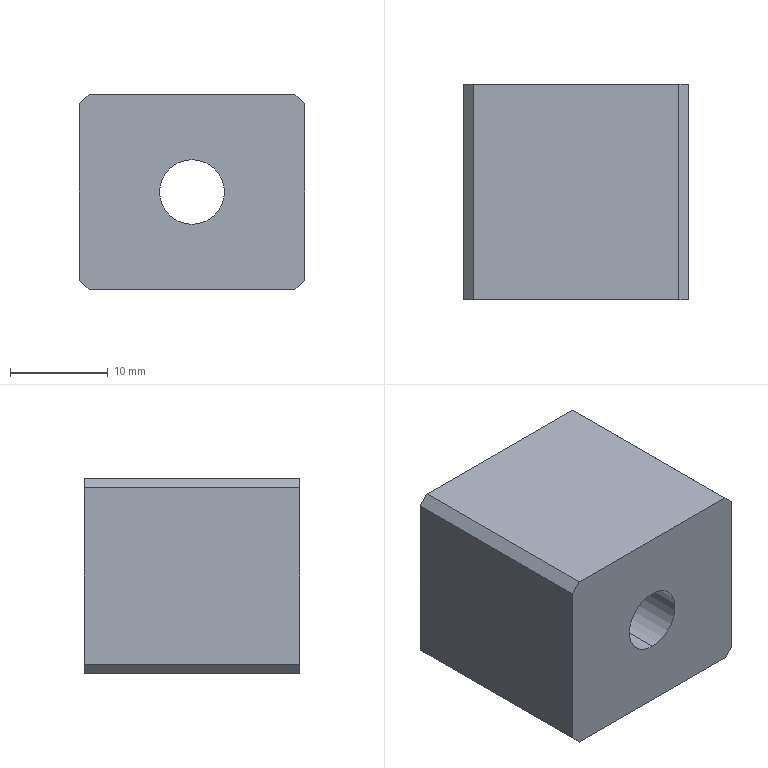Part | SolidWorks | features Chamfer 1, Extrusion 1, HoleWzd 1 | 1 solid | 15 faces | box 23 x 22 x 20 mm | volume 8934 mm3 | plane 11 | cylinder 4 | commonest cylinder face diameters 6.6 x2 11 x2
STEP:
#1=CARTESIAN_POINT('',(0.,4.6,-5.5));
#2=VERTEX_POINT('',#1);
#3=CARTESIAN_POINT('',(0.,4.6,5.5));
#4=VERTEX_POINT('',#3);
#5=CARTESIAN_POINT('',(0.,4.6,0.));
#6=DIRECTION('',(0.,1.,0.));
#7=DIRECTION('',(0.,0.,1.));
#8=AXIS2_PLACEMENT_3D('',#5,#6,#7);
#9=CIRCLE('',#8,5.5);
#10=EDGE_CURVE('',#2,#4,#9,.T.);
#11=ORIENTED_EDGE('',*,*,#10,.F.);
#12=CARTESIAN_POINT('',(0.,11.,-5.5));
#13=VERTEX_POINT('',#12);
#14=CARTESIAN_POINT('',(0.,11.,-5.5));
#15=DIRECTION('',(0.,1.,0.));
#16=VECTOR('',#15,1000.);
#17=LINE('',#14,#16);
#18=EDGE_CURVE('',#2,#13,#17,.T.);
#19=ORIENTED_EDGE('',*,*,#18,.T.);
#20=CARTESIAN_POINT('',(0.,11.,5.5));
#21=VERTEX_POINT('',#20);
#22=CARTESIAN_POINT('',(0.,11.,0.));
#23=DIRECTION('',(0.,1.,0.));
#24=DIRECTION('',(0.,0.,1.));
#25=AXIS2_PLACEMENT_3D('',#22,#23,#24);
#26=CIRCLE('',#25,5.5);
#27=EDGE_CURVE('',#13,#21,#26,.T.);
#28=ORIENTED_EDGE('',*,*,#27,.T.);
#29=CARTESIAN_POINT('',(0.,11.,5.5));
#30=DIRECTION('',(0.,1.,0.));
#31=VECTOR('',#30,1000.);
#32=LINE('',#29,#31);
#33=EDGE_CURVE('',#4,#21,#32,.T.);
#34=ORIENTED_EDGE('',*,*,#33,.F.);
#35=EDGE_LOOP('',(#11,#19,#28,#34));
#36=FACE_OUTER_BOUND('',#35,.T.);
#37=CARTESIAN_POINT('',(0.,11.,0.));
#38=DIRECTION('',(0.,1.,0.));
#39=DIRECTION('',(0.,0.,1.));
#40=AXIS2_PLACEMENT_3D('',#37,#38,#39);
#41=CYLINDRICAL_SURFACE('',#40,5.5);
#42=ADVANCED_FACE('',(#36),#41,.F.);
#43=CARTESIAN_POINT('',(0.,-11.,-3.3));
#44=VERTEX_POINT('',#43);
#45=CARTESIAN_POINT('',(0.,-11.,3.3));
#46=VERTEX_POINT('',#45);
#47=CARTESIAN_POINT('',(0.,-11.,0.));
#48=DIRECTION('',(0.,1.,0.));
#49=DIRECTION('',(0.,0.,1.));
#50=AXIS2_PLACEMENT_3D('',#47,#48,#49);
#51=CIRCLE('',#50,3.3);
#52=EDGE_CURVE('',#44,#46,#51,.T.);
#53=ORIENTED_EDGE('',*,*,#52,.F.);
#54=CARTESIAN_POINT('',(0.,4.6,-3.3));
#55=VERTEX_POINT('',#54);
#56=CARTESIAN_POINT('',(0.,11.,-3.3));
#57=DIRECTION('',(0.,1.,0.));
#58=VECTOR('',#57,1000.);
#59=LINE('',#56,#58);
#60=EDGE_CURVE('',#44,#55,#59,.T.);
#61=ORIENTED_EDGE('',*,*,#60,.T.);
#62=CARTESIAN_POINT('',(0.,4.6,3.3));
#63=VERTEX_POINT('',#62);
#64=CARTESIAN_POINT('',(0.,4.6,0.));
#65=DIRECTION('',(0.,1.,0.));
#66=DIRECTION('',(0.,0.,1.));
#67=AXIS2_PLACEMENT_3D('',#64,#65,#66);
#68=CIRCLE('',#67,3.3);
#69=EDGE_CURVE('',#55,#63,#68,.T.);
#70=ORIENTED_EDGE('',*,*,#69,.T.);
#71=CARTESIAN_POINT('',(0.,11.,3.3));
#72=DIRECTION('',(0.,1.,0.));
#73=VECTOR('',#72,1000.);
#74=LINE('',#71,#73);
#75=EDGE_CURVE('',#46,#63,#74,.T.);
#76=ORIENTED_EDGE('',*,*,#75,.F.);
#77=EDGE_LOOP('',(#53,#61,#70,#76));
#78=FACE_OUTER_BOUND('',#77,.T.);
#79=CARTESIAN_POINT('',(0.,11.,0.));
#80=DIRECTION('',(0.,1.,0.));
#81=DIRECTION('',(0.,0.,1.));
#82=AXIS2_PLACEMENT_3D('',#79,#80,#81);
#83=CYLINDRICAL_SURFACE('',#82,3.3);
#84=ADVANCED_FACE('',(#78),#83,.F.);
#85=CARTESIAN_POINT('',(-11.5,-11.,-9.));
#86=VERTEX_POINT('',#85);
#87=CARTESIAN_POINT('',(-11.5,-11.,9.));
#88=VERTEX_POINT('',#87);
#89=CARTESIAN_POINT('',(-11.5,-11.,-10.));
#90=DIRECTION('',(0.,0.,1.));
#91=VECTOR('',#90,1000.);
#92=LINE('',#89,#91);
#93=EDGE_CURVE('',#86,#88,#92,.T.);
#94=ORIENTED_EDGE('',*,*,#93,.T.);
#95=CARTESIAN_POINT('',(-11.5,11.,9.));
#96=VERTEX_POINT('',#95);
#97=CARTESIAN_POINT('',(-11.5,11.,9.));
#98=DIRECTION('',(0.,1.,0.));
#99=VECTOR('',#98,1000.);
#100=LINE('',#97,#99);
#101=EDGE_CURVE('',#88,#96,#100,.T.);
#102=ORIENTED_EDGE('',*,*,#101,.T.);
#103=CARTESIAN_POINT('',(-11.5,11.,-9.));
#104=VERTEX_POINT('',#103);
#105=CARTESIAN_POINT('',(-11.5,11.,-10.));
#106=DIRECTION('',(0.,0.,1.));
#107=VECTOR('',#106,1000.);
#108=LINE('',#105,#107);
#109=EDGE_CURVE('',#104,#96,#108,.T.);
#110=ORIENTED_EDGE('',*,*,#109,.F.);
#111=CARTESIAN_POINT('',(-11.5,11.,-9.));
#112=DIRECTION('',(0.,-1.,0.));
#113=VECTOR('',#112,1000.);
#114=LINE('',#111,#113);
#115=EDGE_CURVE('',#104,#86,#114,.T.);
#116=ORIENTED_EDGE('',*,*,#115,.T.);
#117=EDGE_LOOP('',(#94,#102,#110,#116));
#118=FACE_OUTER_BOUND('',#117,.T.);
#119=CARTESIAN_POINT('',(-11.5,11.,-10.));
#120=DIRECTION('',(1.,0.,0.));
#121=DIRECTION('',(0.,0.,-1.));
#122=AXIS2_PLACEMENT_3D('',#119,#120,#121);
#123=PLANE('',#122);
#124=ADVANCED_FACE('',(#118),#123,.F.);
#125=CARTESIAN_POINT('',(-10.5,-11.,10.));
#126=VERTEX_POINT('',#125);
#127=CARTESIAN_POINT('',(10.5,-11.,10.));
#128=VERTEX_POINT('',#127);
#129=CARTESIAN_POINT('',(-11.5,-11.,10.));
#130=DIRECTION('',(1.,0.,0.));
#131=VECTOR('',#130,1000.);
#132=LINE('',#129,#131);
#133=EDGE_CURVE('',#126,#128,#132,.T.);
#134=ORIENTED_EDGE('',*,*,#133,.T.);
#135=CARTESIAN_POINT('',(10.5,11.,10.));
#136=VERTEX_POINT('',#135);
#137=CARTESIAN_POINT('',(10.5,11.,10.));
#138=DIRECTION('',(0.,1.,0.));
#139=VECTOR('',#138,1000.);
#140=LINE('',#137,#139);
#141=EDGE_CURVE('',#128,#136,#140,.T.);
#142=ORIENTED_EDGE('',*,*,#141,.T.);
#143=CARTESIAN_POINT('',(-10.5,11.,10.));
#144=VERTEX_POINT('',#143);
#145=CARTESIAN_POINT('',(-11.5,11.,10.));
#146=DIRECTION('',(1.,0.,0.));
#147=VECTOR('',#146,1000.);
#148=LINE('',#145,#147);
#149=EDGE_CURVE('',#144,#136,#148,.T.);
#150=ORIENTED_EDGE('',*,*,#149,.F.);
#151=CARTESIAN_POINT('',(-10.5,11.,10.));
#152=DIRECTION('',(0.,-1.,0.));
#153=VECTOR('',#152,1000.);
#154=LINE('',#151,#153);
#155=EDGE_CURVE('',#144,#126,#154,.T.);
#156=ORIENTED_EDGE('',*,*,#155,.T.);
#157=EDGE_LOOP('',(#134,#142,#150,#156));
#158=FACE_OUTER_BOUND('',#157,.T.);
#159=CARTESIAN_POINT('',(-11.5,11.,10.));
#160=DIRECTION('',(0.,0.,-1.));
#161=DIRECTION('',(-1.,0.,0.));
#162=AXIS2_PLACEMENT_3D('',#159,#160,#161);
#163=PLANE('',#162);
#164=ADVANCED_FACE('',(#158),#163,.F.);
#165=CARTESIAN_POINT('',(11.5,11.,9.));
#166=VERTEX_POINT('',#165);
#167=CARTESIAN_POINT('',(11.5,11.,-9.));
#168=VERTEX_POINT('',#167);
#169=CARTESIAN_POINT('',(11.5,11.,-10.));
#170=DIRECTION('',(0.,0.,-1.));
#171=VECTOR('',#170,1000.);
#172=LINE('',#169,#171);
#173=EDGE_CURVE('',#166,#168,#172,.T.);
#174=ORIENTED_EDGE('',*,*,#173,.F.);
#175=CARTESIAN_POINT('',(11.5,-11.,9.));
#176=VERTEX_POINT('',#175);
#177=CARTESIAN_POINT('',(11.5,11.,9.));
#178=DIRECTION('',(0.,-1.,0.));
#179=VECTOR('',#178,1000.);
#180=LINE('',#177,#179);
#181=EDGE_CURVE('',#166,#176,#180,.T.);
#182=ORIENTED_EDGE('',*,*,#181,.T.);
#183=CARTESIAN_POINT('',(11.5,-11.,-9.));
#184=VERTEX_POINT('',#183);
#185=CARTESIAN_POINT('',(11.5,-11.,-10.));
#186=DIRECTION('',(0.,0.,-1.));
#187=VECTOR('',#186,1000.);
#188=LINE('',#185,#187);
#189=EDGE_CURVE('',#176,#184,#188,.T.);
#190=ORIENTED_EDGE('',*,*,#189,.T.);
#191=CARTESIAN_POINT('',(11.5,11.,-9.));
#192=DIRECTION('',(0.,1.,0.));
#193=VECTOR('',#192,1000.);
#194=LINE('',#191,#193);
#195=EDGE_CURVE('',#184,#168,#194,.T.);
#196=ORIENTED_EDGE('',*,*,#195,.T.);
#197=EDGE_LOOP('',(#174,#182,#190,#196));
#198=FACE_OUTER_BOUND('',#197,.T.);
#199=CARTESIAN_POINT('',(11.5,11.,-10.));
#200=DIRECTION('',(-1.,0.,0.));
#201=DIRECTION('',(0.,0.,1.));
#202=AXIS2_PLACEMENT_3D('',#199,#200,#201);
#203=PLANE('',#202);
#204=ADVANCED_FACE('',(#198),#203,.F.);
#205=CARTESIAN_POINT('',(10.5,11.,-10.));
#206=VERTEX_POINT('',#205);
#207=CARTESIAN_POINT('',(-10.5,11.,-10.));
#208=VERTEX_POINT('',#207);
#209=CARTESIAN_POINT('',(-11.5,11.,-10.));
#210=DIRECTION('',(-1.,0.,0.));
#211=VECTOR('',#210,1000.);
#212=LINE('',#209,#211);
#213=EDGE_CURVE('',#206,#208,#212,.T.);
#214=ORIENTED_EDGE('',*,*,#213,.F.);
#215=CARTESIAN_POINT('',(10.5,-11.,-10.));
#216=VERTEX_POINT('',#215);
#217=CARTESIAN_POINT('',(10.5,11.,-10.));
#218=DIRECTION('',(0.,-1.,0.));
#219=VECTOR('',#218,1000.);
#220=LINE('',#217,#219);
#221=EDGE_CURVE('',#206,#216,#220,.T.);
#222=ORIENTED_EDGE('',*,*,#221,.T.);
#223=CARTESIAN_POINT('',(-10.5,-11.,-10.));
#224=VERTEX_POINT('',#223);
#225=CARTESIAN_POINT('',(-11.5,-11.,-10.));
#226=DIRECTION('',(-1.,0.,0.));
#227=VECTOR('',#226,1000.);
#228=LINE('',#225,#227);
#229=EDGE_CURVE('',#216,#224,#228,.T.);
#230=ORIENTED_EDGE('',*,*,#229,.T.);
#231=CARTESIAN_POINT('',(-10.5,11.,-10.));
#232=DIRECTION('',(0.,1.,0.));
#233=VECTOR('',#232,1000.);
#234=LINE('',#231,#233);
#235=EDGE_CURVE('',#224,#208,#234,.T.);
#236=ORIENTED_EDGE('',*,*,#235,.T.);
#237=EDGE_LOOP('',(#214,#222,#230,#236));
#238=FACE_OUTER_BOUND('',#237,.T.);
#239=CARTESIAN_POINT('',(-11.5,11.,-10.));
#240=DIRECTION('',(0.,0.,1.));
#241=DIRECTION('',(1.,0.,0.));
#242=AXIS2_PLACEMENT_3D('',#239,#240,#241);
#243=PLANE('',#242);
#244=ADVANCED_FACE('',(#238),#243,.F.);
#245=CARTESIAN_POINT('',(0.,11.,0.));
#246=DIRECTION('',(0.,1.,0.));
#247=DIRECTION('',(0.,0.,1.));
#248=AXIS2_PLACEMENT_3D('',#245,#246,#247);
#249=CIRCLE('',#248,5.5);
#250=EDGE_CURVE('',#21,#13,#249,.T.);
#251=ORIENTED_EDGE('',*,*,#250,.F.);
#252=ORIENTED_EDGE('',*,*,#27,.F.);
#253=EDGE_LOOP('',(#251,#252));
#254=FACE_BOUND('',#253,.T.);
#255=ORIENTED_EDGE('',*,*,#149,.T.);
#256=CARTESIAN_POINT('',(10.25,11.,10.25));
#257=DIRECTION('',(0.7071,0.,-0.7071));
#258=VECTOR('',#257,1000.);
#259=LINE('',#256,#258);
#260=EDGE_CURVE('',#136,#166,#259,.T.);
#261=ORIENTED_EDGE('',*,*,#260,.T.);
#262=ORIENTED_EDGE('',*,*,#173,.T.);
#263=CARTESIAN_POINT('',(10.25,11.,-10.25));
#264=DIRECTION('',(-0.7071,0.,-0.7071));
#265=VECTOR('',#264,1000.);
#266=LINE('',#263,#265);
#267=EDGE_CURVE('',#168,#206,#266,.T.);
#268=ORIENTED_EDGE('',*,*,#267,.T.);
#269=ORIENTED_EDGE('',*,*,#213,.T.);
#270=CARTESIAN_POINT('',(-10.25,11.,-10.25));
#271=DIRECTION('',(-0.7071,0.,0.7071));
#272=VECTOR('',#271,1000.);
#273=LINE('',#270,#272);
#274=EDGE_CURVE('',#208,#104,#273,.T.);
#275=ORIENTED_EDGE('',*,*,#274,.T.);
#276=ORIENTED_EDGE('',*,*,#109,.T.);
#277=CARTESIAN_POINT('',(-10.25,11.,10.25));
#278=DIRECTION('',(0.7071,0.,0.7071));
#279=VECTOR('',#278,1000.);
#280=LINE('',#277,#279);
#281=EDGE_CURVE('',#96,#144,#280,.T.);
#282=ORIENTED_EDGE('',*,*,#281,.T.);
#283=EDGE_LOOP('',(#255,#261,#262,#268,#269,#275,#276,#282));
#284=FACE_OUTER_BOUND('',#283,.T.);
#285=CARTESIAN_POINT('',(0.,11.,0.));
#286=DIRECTION('',(0.,1.,0.));
#287=DIRECTION('',(0.,0.,1.));
#288=AXIS2_PLACEMENT_3D('',#285,#286,#287);
#289=PLANE('',#288);
#290=ADVANCED_FACE('',(#254,#284),#289,.T.);
#291=CARTESIAN_POINT('',(0.,-11.,0.));
#292=DIRECTION('',(0.,1.,0.));
#293=DIRECTION('',(0.,0.,1.));
#294=AXIS2_PLACEMENT_3D('',#291,#292,#293);
#295=CIRCLE('',#294,3.3);
#296=EDGE_CURVE('',#46,#44,#295,.T.);
#297=ORIENTED_EDGE('',*,*,#296,.T.);
#298=ORIENTED_EDGE('',*,*,#52,.T.);
#299=EDGE_LOOP('',(#297,#298));
#300=FACE_BOUND('',#299,.T.);
#301=ORIENTED_EDGE('',*,*,#189,.F.);
#302=CARTESIAN_POINT('',(11.5,-11.,9.));
#303=DIRECTION('',(-0.7071,0.,0.7071));
#304=VECTOR('',#303,1000.);
#305=LINE('',#302,#304);
#306=EDGE_CURVE('',#176,#128,#305,.T.);
#307=ORIENTED_EDGE('',*,*,#306,.T.);
#308=ORIENTED_EDGE('',*,*,#133,.F.);
#309=CARTESIAN_POINT('',(-10.5,-11.,10.));
#310=DIRECTION('',(-0.7071,0.,-0.7071));
#311=VECTOR('',#310,1000.);
#312=LINE('',#309,#311);
#313=EDGE_CURVE('',#126,#88,#312,.T.);
#314=ORIENTED_EDGE('',*,*,#313,.T.);
#315=ORIENTED_EDGE('',*,*,#93,.F.);
#316=CARTESIAN_POINT('',(-11.5,-11.,-9.));
#317=DIRECTION('',(0.7071,0.,-0.7071));
#318=VECTOR('',#317,1000.);
#319=LINE('',#316,#318);
#320=EDGE_CURVE('',#86,#224,#319,.T.);
#321=ORIENTED_EDGE('',*,*,#320,.T.);
#322=ORIENTED_EDGE('',*,*,#229,.F.);
#323=CARTESIAN_POINT('',(10.5,-11.,-10.));
#324=DIRECTION('',(0.7071,0.,0.7071));
#325=VECTOR('',#324,1000.);
#326=LINE('',#323,#325);
#327=EDGE_CURVE('',#216,#184,#326,.T.);
#328=ORIENTED_EDGE('',*,*,#327,.T.);
#329=EDGE_LOOP('',(#301,#307,#308,#314,#315,#321,#322,#328));
#330=FACE_OUTER_BOUND('',#329,.T.);
#331=CARTESIAN_POINT('',(0.,-11.,0.));
#332=DIRECTION('',(0.,1.,0.));
#333=DIRECTION('',(0.,0.,1.));
#334=AXIS2_PLACEMENT_3D('',#331,#332,#333);
#335=PLANE('',#334);
#336=ADVANCED_FACE('',(#300,#330),#335,.F.);
#337=ORIENTED_EDGE('',*,*,#60,.F.);
#338=ORIENTED_EDGE('',*,*,#296,.F.);
#339=ORIENTED_EDGE('',*,*,#75,.T.);
#340=CARTESIAN_POINT('',(0.,4.6,0.));
#341=DIRECTION('',(0.,1.,0.));
#342=DIRECTION('',(0.,0.,1.));
#343=AXIS2_PLACEMENT_3D('',#340,#341,#342);
#344=CIRCLE('',#343,3.3);
#345=EDGE_CURVE('',#63,#55,#344,.T.);
#346=ORIENTED_EDGE('',*,*,#345,.T.);
#347=EDGE_LOOP('',(#337,#338,#339,#346));
#348=FACE_OUTER_BOUND('',#347,.T.);
#349=CARTESIAN_POINT('',(0.,11.,0.));
#350=DIRECTION('',(0.,1.,0.));
#351=DIRECTION('',(0.,0.,1.));
#352=AXIS2_PLACEMENT_3D('',#349,#350,#351);
#353=CYLINDRICAL_SURFACE('',#352,3.3);
#354=ADVANCED_FACE('',(#348),#353,.F.);
#355=ORIENTED_EDGE('',*,*,#345,.F.);
#356=ORIENTED_EDGE('',*,*,#69,.F.);
#357=EDGE_LOOP('',(#355,#356));
#358=FACE_BOUND('',#357,.T.);
#359=CARTESIAN_POINT('',(0.,4.6,0.));
#360=DIRECTION('',(0.,1.,0.));
#361=DIRECTION('',(0.,0.,1.));
#362=AXIS2_PLACEMENT_3D('',#359,#360,#361);
#363=CIRCLE('',#362,5.5);
#364=EDGE_CURVE('',#4,#2,#363,.T.);
#365=ORIENTED_EDGE('',*,*,#364,.T.);
#366=ORIENTED_EDGE('',*,*,#10,.T.);
#367=EDGE_LOOP('',(#365,#366));
#368=FACE_OUTER_BOUND('',#367,.T.);
#369=CARTESIAN_POINT('',(3.3,4.6,0.));
#370=DIRECTION('',(0.,-1.,0.));
#371=DIRECTION('',(0.,0.,-1.));
#372=AXIS2_PLACEMENT_3D('',#369,#370,#371);
#373=PLANE('',#372);
#374=ADVANCED_FACE('',(#358,#368),#373,.F.);
#375=ORIENTED_EDGE('',*,*,#18,.F.);
#376=ORIENTED_EDGE('',*,*,#364,.F.);
#377=ORIENTED_EDGE('',*,*,#33,.T.);
#378=ORIENTED_EDGE('',*,*,#250,.T.);
#379=EDGE_LOOP('',(#375,#376,#377,#378));
#380=FACE_OUTER_BOUND('',#379,.T.);
#381=CARTESIAN_POINT('',(0.,11.,0.));
#382=DIRECTION('',(0.,1.,0.));
#383=DIRECTION('',(0.,0.,1.));
#384=AXIS2_PLACEMENT_3D('',#381,#382,#383);
#385=CYLINDRICAL_SURFACE('',#384,5.5);
#386=ADVANCED_FACE('',(#380),#385,.F.);
#387=ORIENTED_EDGE('',*,*,#260,.F.);
#388=ORIENTED_EDGE('',*,*,#141,.F.);
#389=ORIENTED_EDGE('',*,*,#306,.F.);
#390=ORIENTED_EDGE('',*,*,#181,.F.);
#391=EDGE_LOOP('',(#387,#388,#389,#390));
#392=FACE_OUTER_BOUND('',#391,.T.);
#393=CARTESIAN_POINT('',(11.5,11.,9.));
#394=DIRECTION('',(-0.7071,0.,-0.7071));
#395=DIRECTION('',(0.,-1.,0.));
#396=AXIS2_PLACEMENT_3D('',#393,#394,#395);
#397=PLANE('',#396);
#398=ADVANCED_FACE('',(#392),#397,.F.);
#399=ORIENTED_EDGE('',*,*,#281,.F.);
#400=ORIENTED_EDGE('',*,*,#101,.F.);
#401=ORIENTED_EDGE('',*,*,#313,.F.);
#402=ORIENTED_EDGE('',*,*,#155,.F.);
#403=EDGE_LOOP('',(#399,#400,#401,#402));
#404=FACE_OUTER_BOUND('',#403,.T.);
#405=CARTESIAN_POINT('',(-10.5,11.,10.));
#406=DIRECTION('',(0.7071,0.,-0.7071));
#407=DIRECTION('',(0.,-1.,0.));
#408=AXIS2_PLACEMENT_3D('',#405,#406,#407);
#409=PLANE('',#408);
#410=ADVANCED_FACE('',(#404),#409,.F.);
#411=ORIENTED_EDGE('',*,*,#267,.F.);
#412=ORIENTED_EDGE('',*,*,#195,.F.);
#413=ORIENTED_EDGE('',*,*,#327,.F.);
#414=ORIENTED_EDGE('',*,*,#221,.F.);
#415=EDGE_LOOP('',(#411,#412,#413,#414));
#416=FACE_OUTER_BOUND('',#415,.T.);
#417=CARTESIAN_POINT('',(10.5,11.,-10.));
#418=DIRECTION('',(-0.7071,0.,0.7071));
#419=DIRECTION('',(0.,-1.,0.));
#420=AXIS2_PLACEMENT_3D('',#417,#418,#419);
#421=PLANE('',#420);
#422=ADVANCED_FACE('',(#416),#421,.F.);
#423=ORIENTED_EDGE('',*,*,#274,.F.);
#424=ORIENTED_EDGE('',*,*,#235,.F.);
#425=ORIENTED_EDGE('',*,*,#320,.F.);
#426=ORIENTED_EDGE('',*,*,#115,.F.);
#427=EDGE_LOOP('',(#423,#424,#425,#426));
#428=FACE_OUTER_BOUND('',#427,.T.);
#429=CARTESIAN_POINT('',(-11.5,11.,-9.));
#430=DIRECTION('',(0.7071,0.,0.7071));
#431=DIRECTION('',(0.,-1.,0.));
#432=AXIS2_PLACEMENT_3D('',#429,#430,#431);
#433=PLANE('',#432);
#434=ADVANCED_FACE('',(#428),#433,.F.);
#435=CLOSED_SHELL('',(#42,#84,#124,#164,#204,#244,#290,#336,#354,#374,#386,#398,#410,#422,#434));
#436=MANIFOLD_SOLID_BREP('',#435);
#437=CARTESIAN_POINT('',(0.,0.,0.));
#438=DIRECTION('',(0.,0.,1.));
#439=DIRECTION('',(1.,0.,0.));
#440=AXIS2_PLACEMENT_3D('',#437,#438,#439);
#441=(LENGTH_UNIT()NAMED_UNIT(*)SI_UNIT(.MILLI.,.METRE.));
#442=UNCERTAINTY_MEASURE_WITH_UNIT(LENGTH_MEASURE(0.00001),#441,'','');
#443=(NAMED_UNIT(*)PLANE_ANGLE_UNIT()SI_UNIT($,.RADIAN.));
#444=(NAMED_UNIT(*)SI_UNIT($,.STERADIAN.)SOLID_ANGLE_UNIT());
#445=(GEOMETRIC_REPRESENTATION_CONTEXT(3)GLOBAL_UNCERTAINTY_ASSIGNED_CONTEXT((#442))GLOBAL_UNIT_ASSIGNED_CONTEXT((#441,#443,#444))REPRESENTATION_CONTEXT('',''));
#446=ADVANCED_BREP_SHAPE_REPRESENTATION('',(#436,#440),#445);